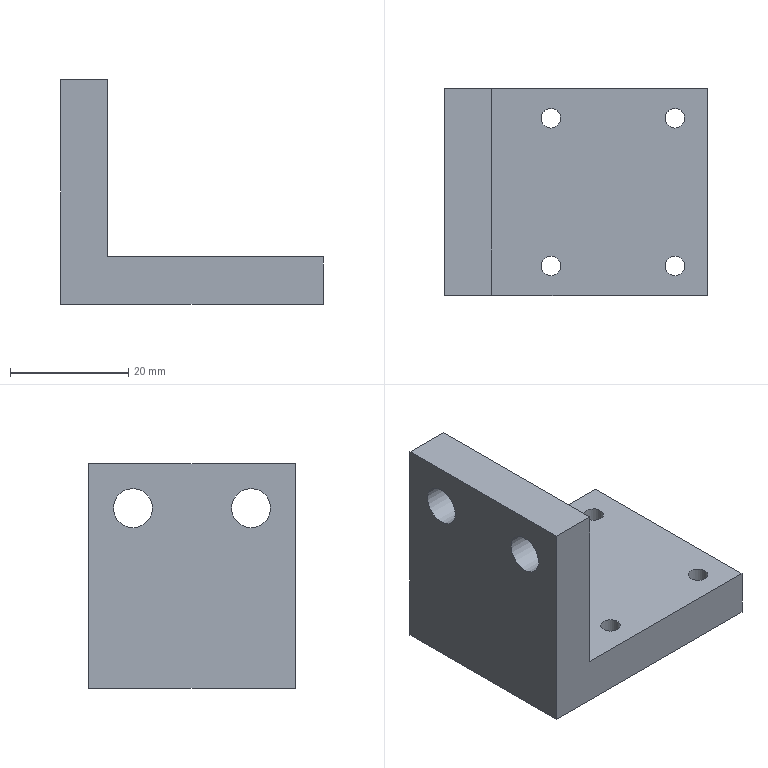Part | NX | features 5003_208_Bracket 2 | 1 solid | 14 faces | box 44.5 x 35 x 38 mm | volume 20039 mm3 | plane 8 | cylinder 6 | commonest cylinder face diameters 3.3 x4 6.6 x2
STEP:
#1=CARTESIAN_POINT('',(195.825,68.05,-119.58));
#2=VERTEX_POINT('',#1);
#3=CARTESIAN_POINT('',(195.825,66.4,-119.58));
#4=DIRECTION('',(0.,0.,1.));
#5=DIRECTION('',(0.,1.,0.));
#6=AXIS2_PLACEMENT_3D('',#3,#4,#5);
#7=CIRCLE('',#6,1.65);
#8=EDGE_CURVE('',#2,#2,#7,.T.);
#9=ORIENTED_EDGE('',*,*,#8,.F.);
#10=EDGE_LOOP('',(#9));
#11=FACE_BOUND('',#10,.T.);
#12=CARTESIAN_POINT('',(195.825,93.05,-119.58));
#13=VERTEX_POINT('',#12);
#14=CARTESIAN_POINT('',(195.825,91.4,-119.58));
#15=DIRECTION('',(0.,0.,1.));
#16=DIRECTION('',(0.,1.,0.));
#17=AXIS2_PLACEMENT_3D('',#14,#15,#16);
#18=CIRCLE('',#17,1.65);
#19=EDGE_CURVE('',#13,#13,#18,.T.);
#20=ORIENTED_EDGE('',*,*,#19,.F.);
#21=EDGE_LOOP('',(#20));
#22=FACE_BOUND('',#21,.T.);
#23=CARTESIAN_POINT('',(216.825,93.05,-119.58));
#24=VERTEX_POINT('',#23);
#25=CARTESIAN_POINT('',(216.825,91.4,-119.58));
#26=DIRECTION('',(0.,0.,1.));
#27=DIRECTION('',(0.,1.,0.));
#28=AXIS2_PLACEMENT_3D('',#25,#26,#27);
#29=CIRCLE('',#28,1.65);
#30=EDGE_CURVE('',#24,#24,#29,.T.);
#31=ORIENTED_EDGE('',*,*,#30,.F.);
#32=EDGE_LOOP('',(#31));
#33=FACE_BOUND('',#32,.T.);
#34=CARTESIAN_POINT('',(216.825,68.05,-119.58));
#35=VERTEX_POINT('',#34);
#36=CARTESIAN_POINT('',(216.825,66.4,-119.58));
#37=DIRECTION('',(0.,0.,1.));
#38=DIRECTION('',(0.,1.,0.));
#39=AXIS2_PLACEMENT_3D('',#36,#37,#38);
#40=CIRCLE('',#39,1.65);
#41=EDGE_CURVE('',#35,#35,#40,.T.);
#42=ORIENTED_EDGE('',*,*,#41,.F.);
#43=EDGE_LOOP('',(#42));
#44=FACE_BOUND('',#43,.T.);
#45=CARTESIAN_POINT('',(185.825,61.4,-119.58));
#46=VERTEX_POINT('',#45);
#47=CARTESIAN_POINT('',(185.825,96.4,-119.58));
#48=VERTEX_POINT('',#47);
#49=CARTESIAN_POINT('',(185.825,96.4,-119.58));
#50=DIRECTION('',(0.,1.,0.));
#51=VECTOR('',#50,1000.);
#52=LINE('',#49,#51);
#53=EDGE_CURVE('',#46,#48,#52,.T.);
#54=ORIENTED_EDGE('',*,*,#53,.F.);
#55=CARTESIAN_POINT('',(222.325,61.4,-119.58));
#56=VERTEX_POINT('',#55);
#57=CARTESIAN_POINT('',(177.825,61.4,-119.58));
#58=DIRECTION('',(-1.,0.,0.));
#59=VECTOR('',#58,1000.);
#60=LINE('',#57,#59);
#61=EDGE_CURVE('',#56,#46,#60,.T.);
#62=ORIENTED_EDGE('',*,*,#61,.F.);
#63=CARTESIAN_POINT('',(222.325,96.4,-119.58));
#64=VERTEX_POINT('',#63);
#65=CARTESIAN_POINT('',(222.325,96.4,-119.58));
#66=DIRECTION('',(0.,-1.,0.));
#67=VECTOR('',#66,1000.);
#68=LINE('',#65,#67);
#69=EDGE_CURVE('',#64,#56,#68,.T.);
#70=ORIENTED_EDGE('',*,*,#69,.F.);
#71=CARTESIAN_POINT('',(177.825,96.4,-119.58));
#72=DIRECTION('',(1.,0.,0.));
#73=VECTOR('',#72,1000.);
#74=LINE('',#71,#73);
#75=EDGE_CURVE('',#48,#64,#74,.T.);
#76=ORIENTED_EDGE('',*,*,#75,.F.);
#77=EDGE_LOOP('',(#54,#62,#70,#76));
#78=FACE_BOUND('',#77,.T.);
#79=CARTESIAN_POINT('',(-28.104,149.362,-119.58));
#80=DIRECTION('',(0.,0.,-1.));
#81=DIRECTION('',(0.,-1.,0.));
#82=AXIS2_PLACEMENT_3D('',#79,#80,#81);
#83=PLANE('',#82);
#84=ADVANCED_FACE('',(#11,#22,#33,#44,#78),#83,.F.);
#85=CARTESIAN_POINT('',(177.825,96.4,-127.58));
#86=VERTEX_POINT('',#85);
#87=CARTESIAN_POINT('',(177.825,96.4,-89.58));
#88=VERTEX_POINT('',#87);
#89=CARTESIAN_POINT('',(177.825,96.4,-127.58));
#90=DIRECTION('',(0.,0.,1.));
#91=VECTOR('',#90,1000.);
#92=LINE('',#89,#91);
#93=EDGE_CURVE('',#86,#88,#92,.T.);
#94=ORIENTED_EDGE('',*,*,#93,.T.);
#95=CARTESIAN_POINT('',(185.825,96.4,-89.58));
#96=VERTEX_POINT('',#95);
#97=CARTESIAN_POINT('',(177.825,96.4,-89.58));
#98=DIRECTION('',(-1.,0.,0.));
#99=VECTOR('',#98,1000.);
#100=LINE('',#97,#99);
#101=EDGE_CURVE('',#96,#88,#100,.T.);
#102=ORIENTED_EDGE('',*,*,#101,.F.);
#103=CARTESIAN_POINT('',(185.825,96.4,-89.58));
#104=DIRECTION('',(0.,0.,-1.));
#105=VECTOR('',#104,1000.);
#106=LINE('',#103,#105);
#107=EDGE_CURVE('',#96,#48,#106,.T.);
#108=ORIENTED_EDGE('',*,*,#107,.T.);
#109=ORIENTED_EDGE('',*,*,#75,.T.);
#110=CARTESIAN_POINT('',(222.325,96.4,-127.58));
#111=VERTEX_POINT('',#110);
#112=CARTESIAN_POINT('',(222.325,96.4,-127.58));
#113=DIRECTION('',(0.,0.,1.));
#114=VECTOR('',#113,1000.);
#115=LINE('',#112,#114);
#116=EDGE_CURVE('',#111,#64,#115,.T.);
#117=ORIENTED_EDGE('',*,*,#116,.F.);
#118=CARTESIAN_POINT('',(177.825,96.4,-127.58));
#119=DIRECTION('',(1.,0.,0.));
#120=VECTOR('',#119,1000.);
#121=LINE('',#118,#120);
#122=EDGE_CURVE('',#86,#111,#121,.T.);
#123=ORIENTED_EDGE('',*,*,#122,.F.);
#124=EDGE_LOOP('',(#94,#102,#108,#109,#117,#123));
#125=FACE_BOUND('',#124,.T.);
#126=CARTESIAN_POINT('',(177.825,96.4,-127.58));
#127=DIRECTION('',(0.,-1.,0.));
#128=DIRECTION('',(0.,0.,1.));
#129=AXIS2_PLACEMENT_3D('',#126,#127,#128);
#130=PLANE('',#129);
#131=ADVANCED_FACE('',(#125),#130,.F.);
#132=ORIENTED_EDGE('',*,*,#69,.T.);
#133=CARTESIAN_POINT('',(222.325,61.4,-127.58));
#134=VERTEX_POINT('',#133);
#135=CARTESIAN_POINT('',(222.325,61.4,-127.58));
#136=DIRECTION('',(0.,0.,1.));
#137=VECTOR('',#136,1000.);
#138=LINE('',#135,#137);
#139=EDGE_CURVE('',#134,#56,#138,.T.);
#140=ORIENTED_EDGE('',*,*,#139,.F.);
#141=CARTESIAN_POINT('',(222.325,96.4,-127.58));
#142=DIRECTION('',(0.,-1.,0.));
#143=VECTOR('',#142,1000.);
#144=LINE('',#141,#143);
#145=EDGE_CURVE('',#111,#134,#144,.T.);
#146=ORIENTED_EDGE('',*,*,#145,.F.);
#147=ORIENTED_EDGE('',*,*,#116,.T.);
#148=EDGE_LOOP('',(#132,#140,#146,#147));
#149=FACE_BOUND('',#148,.T.);
#150=CARTESIAN_POINT('',(222.325,96.4,-127.58));
#151=DIRECTION('',(-1.,0.,0.));
#152=DIRECTION('',(0.,0.,-1.));
#153=AXIS2_PLACEMENT_3D('',#150,#151,#152);
#154=PLANE('',#153);
#155=ADVANCED_FACE('',(#149),#154,.F.);
#156=ORIENTED_EDGE('',*,*,#61,.T.);
#157=CARTESIAN_POINT('',(185.825,61.4,-89.58));
#158=VERTEX_POINT('',#157);
#159=CARTESIAN_POINT('',(185.825,61.4,-89.58));
#160=DIRECTION('',(0.,0.,-1.));
#161=VECTOR('',#160,1000.);
#162=LINE('',#159,#161);
#163=EDGE_CURVE('',#158,#46,#162,.T.);
#164=ORIENTED_EDGE('',*,*,#163,.F.);
#165=CARTESIAN_POINT('',(177.825,61.4,-89.58));
#166=VERTEX_POINT('',#165);
#167=CARTESIAN_POINT('',(177.825,61.4,-89.58));
#168=DIRECTION('',(1.,0.,0.));
#169=VECTOR('',#168,1000.);
#170=LINE('',#167,#169);
#171=EDGE_CURVE('',#166,#158,#170,.T.);
#172=ORIENTED_EDGE('',*,*,#171,.F.);
#173=CARTESIAN_POINT('',(177.825,61.4,-127.58));
#174=VERTEX_POINT('',#173);
#175=CARTESIAN_POINT('',(177.825,61.4,-127.58));
#176=DIRECTION('',(0.,0.,1.));
#177=VECTOR('',#176,1000.);
#178=LINE('',#175,#177);
#179=EDGE_CURVE('',#174,#166,#178,.T.);
#180=ORIENTED_EDGE('',*,*,#179,.F.);
#181=CARTESIAN_POINT('',(177.825,61.4,-127.58));
#182=DIRECTION('',(-1.,0.,0.));
#183=VECTOR('',#182,1000.);
#184=LINE('',#181,#183);
#185=EDGE_CURVE('',#134,#174,#184,.T.);
#186=ORIENTED_EDGE('',*,*,#185,.F.);
#187=ORIENTED_EDGE('',*,*,#139,.T.);
#188=EDGE_LOOP('',(#156,#164,#172,#180,#186,#187));
#189=FACE_BOUND('',#188,.T.);
#190=CARTESIAN_POINT('',(177.825,61.4,-127.58));
#191=DIRECTION('',(0.,1.,0.));
#192=DIRECTION('',(0.,0.,-1.));
#193=AXIS2_PLACEMENT_3D('',#190,#191,#192);
#194=PLANE('',#193);
#195=ADVANCED_FACE('',(#189),#194,.F.);
#196=CARTESIAN_POINT('',(177.825,88.9,-100.38));
#197=VERTEX_POINT('',#196);
#198=CARTESIAN_POINT('',(177.825,88.9,-97.08));
#199=DIRECTION('',(-1.,0.,0.));
#200=DIRECTION('',(0.,0.,-1.));
#201=AXIS2_PLACEMENT_3D('',#198,#199,#200);
#202=CIRCLE('',#201,3.3);
#203=EDGE_CURVE('',#197,#197,#202,.T.);
#204=ORIENTED_EDGE('',*,*,#203,.F.);
#205=EDGE_LOOP('',(#204));
#206=FACE_BOUND('',#205,.T.);
#207=CARTESIAN_POINT('',(177.825,68.9,-100.38));
#208=VERTEX_POINT('',#207);
#209=CARTESIAN_POINT('',(177.825,68.9,-97.08));
#210=DIRECTION('',(-1.,0.,0.));
#211=DIRECTION('',(0.,0.,-1.));
#212=AXIS2_PLACEMENT_3D('',#209,#210,#211);
#213=CIRCLE('',#212,3.3);
#214=EDGE_CURVE('',#208,#208,#213,.T.);
#215=ORIENTED_EDGE('',*,*,#214,.F.);
#216=EDGE_LOOP('',(#215));
#217=FACE_BOUND('',#216,.T.);
#218=ORIENTED_EDGE('',*,*,#179,.T.);
#219=CARTESIAN_POINT('',(177.825,96.4,-89.58));
#220=DIRECTION('',(0.,-1.,0.));
#221=VECTOR('',#220,1000.);
#222=LINE('',#219,#221);
#223=EDGE_CURVE('',#88,#166,#222,.T.);
#224=ORIENTED_EDGE('',*,*,#223,.F.);
#225=ORIENTED_EDGE('',*,*,#93,.F.);
#226=CARTESIAN_POINT('',(177.825,96.4,-127.58));
#227=DIRECTION('',(0.,1.,0.));
#228=VECTOR('',#227,1000.);
#229=LINE('',#226,#228);
#230=EDGE_CURVE('',#174,#86,#229,.T.);
#231=ORIENTED_EDGE('',*,*,#230,.F.);
#232=EDGE_LOOP('',(#218,#224,#225,#231));
#233=FACE_BOUND('',#232,.T.);
#234=CARTESIAN_POINT('',(177.825,96.4,-127.58));
#235=DIRECTION('',(1.,0.,0.));
#236=DIRECTION('',(0.,0.,1.));
#237=AXIS2_PLACEMENT_3D('',#234,#235,#236);
#238=PLANE('',#237);
#239=ADVANCED_FACE('',(#206,#217,#233),#238,.F.);
#240=CARTESIAN_POINT('',(216.825,68.05,-127.58));
#241=VERTEX_POINT('',#240);
#242=CARTESIAN_POINT('',(216.825,66.4,-127.58));
#243=DIRECTION('',(0.,0.,1.));
#244=DIRECTION('',(0.,1.,0.));
#245=AXIS2_PLACEMENT_3D('',#242,#243,#244);
#246=CIRCLE('',#245,1.65);
#247=EDGE_CURVE('',#241,#241,#246,.T.);
#248=ORIENTED_EDGE('',*,*,#247,.T.);
#249=EDGE_LOOP('',(#248));
#250=FACE_BOUND('',#249,.T.);
#251=CARTESIAN_POINT('',(216.825,93.05,-127.58));
#252=VERTEX_POINT('',#251);
#253=CARTESIAN_POINT('',(216.825,91.4,-127.58));
#254=DIRECTION('',(0.,0.,1.));
#255=DIRECTION('',(0.,1.,0.));
#256=AXIS2_PLACEMENT_3D('',#253,#254,#255);
#257=CIRCLE('',#256,1.65);
#258=EDGE_CURVE('',#252,#252,#257,.T.);
#259=ORIENTED_EDGE('',*,*,#258,.T.);
#260=EDGE_LOOP('',(#259));
#261=FACE_BOUND('',#260,.T.);
#262=CARTESIAN_POINT('',(195.825,93.05,-127.58));
#263=VERTEX_POINT('',#262);
#264=CARTESIAN_POINT('',(195.825,91.4,-127.58));
#265=DIRECTION('',(0.,0.,1.));
#266=DIRECTION('',(0.,1.,0.));
#267=AXIS2_PLACEMENT_3D('',#264,#265,#266);
#268=CIRCLE('',#267,1.65);
#269=EDGE_CURVE('',#263,#263,#268,.T.);
#270=ORIENTED_EDGE('',*,*,#269,.T.);
#271=EDGE_LOOP('',(#270));
#272=FACE_BOUND('',#271,.T.);
#273=CARTESIAN_POINT('',(195.825,68.05,-127.58));
#274=VERTEX_POINT('',#273);
#275=CARTESIAN_POINT('',(195.825,66.4,-127.58));
#276=DIRECTION('',(0.,0.,1.));
#277=DIRECTION('',(0.,1.,0.));
#278=AXIS2_PLACEMENT_3D('',#275,#276,#277);
#279=CIRCLE('',#278,1.65);
#280=EDGE_CURVE('',#274,#274,#279,.T.);
#281=ORIENTED_EDGE('',*,*,#280,.T.);
#282=EDGE_LOOP('',(#281));
#283=FACE_BOUND('',#282,.T.);
#284=ORIENTED_EDGE('',*,*,#122,.T.);
#285=ORIENTED_EDGE('',*,*,#145,.T.);
#286=ORIENTED_EDGE('',*,*,#185,.T.);
#287=ORIENTED_EDGE('',*,*,#230,.T.);
#288=EDGE_LOOP('',(#284,#285,#286,#287));
#289=FACE_BOUND('',#288,.T.);
#290=CARTESIAN_POINT('',(-28.104,149.362,-127.58));
#291=DIRECTION('',(0.,0.,-1.));
#292=DIRECTION('',(0.,-1.,0.));
#293=AXIS2_PLACEMENT_3D('',#290,#291,#292);
#294=PLANE('',#293);
#295=ADVANCED_FACE('',(#250,#261,#272,#283,#289),#294,.T.);
#296=ORIENTED_EDGE('',*,*,#280,.F.);
#297=EDGE_LOOP('',(#296));
#298=FACE_BOUND('',#297,.T.);
#299=ORIENTED_EDGE('',*,*,#8,.T.);
#300=EDGE_LOOP('',(#299));
#301=FACE_BOUND('',#300,.T.);
#302=CARTESIAN_POINT('',(195.825,66.4,-119.58));
#303=DIRECTION('',(0.,0.,1.));
#304=DIRECTION('',(0.,1.,0.));
#305=AXIS2_PLACEMENT_3D('',#302,#303,#304);
#306=CYLINDRICAL_SURFACE('',#305,1.65);
#307=ADVANCED_FACE('',(#298,#301),#306,.F.);
#308=ORIENTED_EDGE('',*,*,#269,.F.);
#309=EDGE_LOOP('',(#308));
#310=FACE_BOUND('',#309,.T.);
#311=ORIENTED_EDGE('',*,*,#19,.T.);
#312=EDGE_LOOP('',(#311));
#313=FACE_BOUND('',#312,.T.);
#314=CARTESIAN_POINT('',(195.825,91.4,-119.58));
#315=DIRECTION('',(0.,0.,1.));
#316=DIRECTION('',(0.,1.,0.));
#317=AXIS2_PLACEMENT_3D('',#314,#315,#316);
#318=CYLINDRICAL_SURFACE('',#317,1.65);
#319=ADVANCED_FACE('',(#310,#313),#318,.F.);
#320=ORIENTED_EDGE('',*,*,#258,.F.);
#321=EDGE_LOOP('',(#320));
#322=FACE_BOUND('',#321,.T.);
#323=ORIENTED_EDGE('',*,*,#30,.T.);
#324=EDGE_LOOP('',(#323));
#325=FACE_BOUND('',#324,.T.);
#326=CARTESIAN_POINT('',(216.825,91.4,-119.58));
#327=DIRECTION('',(0.,0.,1.));
#328=DIRECTION('',(0.,1.,0.));
#329=AXIS2_PLACEMENT_3D('',#326,#327,#328);
#330=CYLINDRICAL_SURFACE('',#329,1.65);
#331=ADVANCED_FACE('',(#322,#325),#330,.F.);
#332=ORIENTED_EDGE('',*,*,#247,.F.);
#333=EDGE_LOOP('',(#332));
#334=FACE_BOUND('',#333,.T.);
#335=ORIENTED_EDGE('',*,*,#41,.T.);
#336=EDGE_LOOP('',(#335));
#337=FACE_BOUND('',#336,.T.);
#338=CARTESIAN_POINT('',(216.825,66.4,-119.58));
#339=DIRECTION('',(0.,0.,1.));
#340=DIRECTION('',(0.,1.,0.));
#341=AXIS2_PLACEMENT_3D('',#338,#339,#340);
#342=CYLINDRICAL_SURFACE('',#341,1.65);
#343=ADVANCED_FACE('',(#334,#337),#342,.F.);
#344=CARTESIAN_POINT('',(185.825,88.9,-100.38));
#345=VERTEX_POINT('',#344);
#346=CARTESIAN_POINT('',(185.825,88.9,-97.08));
#347=DIRECTION('',(-1.,0.,0.));
#348=DIRECTION('',(0.,0.,-1.));
#349=AXIS2_PLACEMENT_3D('',#346,#347,#348);
#350=CIRCLE('',#349,3.3);
#351=EDGE_CURVE('',#345,#345,#350,.T.);
#352=ORIENTED_EDGE('',*,*,#351,.T.);
#353=EDGE_LOOP('',(#352));
#354=FACE_BOUND('',#353,.T.);
#355=CARTESIAN_POINT('',(185.825,68.9,-100.38));
#356=VERTEX_POINT('',#355);
#357=CARTESIAN_POINT('',(185.825,68.9,-97.08));
#358=DIRECTION('',(-1.,0.,0.));
#359=DIRECTION('',(0.,0.,-1.));
#360=AXIS2_PLACEMENT_3D('',#357,#358,#359);
#361=CIRCLE('',#360,3.3);
#362=EDGE_CURVE('',#356,#356,#361,.T.);
#363=ORIENTED_EDGE('',*,*,#362,.T.);
#364=EDGE_LOOP('',(#363));
#365=FACE_BOUND('',#364,.T.);
#366=ORIENTED_EDGE('',*,*,#53,.T.);
#367=ORIENTED_EDGE('',*,*,#107,.F.);
#368=CARTESIAN_POINT('',(185.825,96.4,-89.58));
#369=DIRECTION('',(0.,1.,0.));
#370=VECTOR('',#369,1000.);
#371=LINE('',#368,#370);
#372=EDGE_CURVE('',#158,#96,#371,.T.);
#373=ORIENTED_EDGE('',*,*,#372,.F.);
#374=ORIENTED_EDGE('',*,*,#163,.T.);
#375=EDGE_LOOP('',(#366,#367,#373,#374));
#376=FACE_BOUND('',#375,.T.);
#377=CARTESIAN_POINT('',(185.825,96.4,-89.58));
#378=DIRECTION('',(-1.,0.,0.));
#379=DIRECTION('',(0.,0.,-1.));
#380=AXIS2_PLACEMENT_3D('',#377,#378,#379);
#381=PLANE('',#380);
#382=ADVANCED_FACE('',(#354,#365,#376),#381,.F.);
#383=ORIENTED_EDGE('',*,*,#101,.T.);
#384=ORIENTED_EDGE('',*,*,#223,.T.);
#385=ORIENTED_EDGE('',*,*,#171,.T.);
#386=ORIENTED_EDGE('',*,*,#372,.T.);
#387=EDGE_LOOP('',(#383,#384,#385,#386));
#388=FACE_BOUND('',#387,.T.);
#389=CARTESIAN_POINT('',(-28.104,149.362,-89.58));
#390=DIRECTION('',(0.,0.,-1.));
#391=DIRECTION('',(0.,-1.,0.));
#392=AXIS2_PLACEMENT_3D('',#389,#390,#391);
#393=PLANE('',#392);
#394=ADVANCED_FACE('',(#388),#393,.F.);
#395=ORIENTED_EDGE('',*,*,#214,.T.);
#396=EDGE_LOOP('',(#395));
#397=FACE_BOUND('',#396,.T.);
#398=ORIENTED_EDGE('',*,*,#362,.F.);
#399=EDGE_LOOP('',(#398));
#400=FACE_BOUND('',#399,.T.);
#401=CARTESIAN_POINT('',(177.825,68.9,-97.08));
#402=DIRECTION('',(-1.,0.,0.));
#403=DIRECTION('',(0.,0.,-1.));
#404=AXIS2_PLACEMENT_3D('',#401,#402,#403);
#405=CYLINDRICAL_SURFACE('',#404,3.3);
#406=ADVANCED_FACE('',(#397,#400),#405,.F.);
#407=ORIENTED_EDGE('',*,*,#203,.T.);
#408=EDGE_LOOP('',(#407));
#409=FACE_BOUND('',#408,.T.);
#410=ORIENTED_EDGE('',*,*,#351,.F.);
#411=EDGE_LOOP('',(#410));
#412=FACE_BOUND('',#411,.T.);
#413=CARTESIAN_POINT('',(177.825,88.9,-97.08));
#414=DIRECTION('',(-1.,0.,0.));
#415=DIRECTION('',(0.,0.,-1.));
#416=AXIS2_PLACEMENT_3D('',#413,#414,#415);
#417=CYLINDRICAL_SURFACE('',#416,3.3);
#418=ADVANCED_FACE('',(#409,#412),#417,.F.);
#419=CLOSED_SHELL('',(#84,#131,#155,#195,#239,#295,#307,#319,#331,#343,#382,#394,#406,#418));
#420=MANIFOLD_SOLID_BREP('',#419);
#421=(LENGTH_UNIT()NAMED_UNIT(*)SI_UNIT(.MILLI.,.METRE.));
#422=UNCERTAINTY_MEASURE_WITH_UNIT(LENGTH_MEASURE(0.00001),#421,'','');
#423=(NAMED_UNIT(*)PLANE_ANGLE_UNIT()SI_UNIT($,.RADIAN.));
#424=(NAMED_UNIT(*)SI_UNIT($,.STERADIAN.)SOLID_ANGLE_UNIT());
#425=(GEOMETRIC_REPRESENTATION_CONTEXT(3)GLOBAL_UNCERTAINTY_ASSIGNED_CONTEXT((#422))GLOBAL_UNIT_ASSIGNED_CONTEXT((#421,#423,#424))REPRESENTATION_CONTEXT('',''));
#426=ADVANCED_BREP_SHAPE_REPRESENTATION('',(#420),#425);